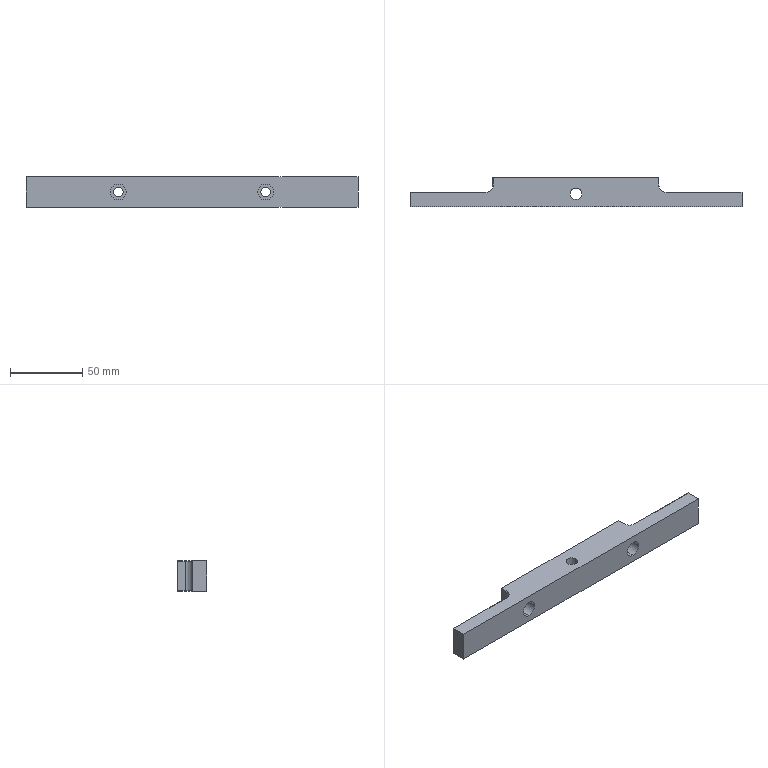Part | STEP file | 调平杆^刮墨刀-350 | 1 solid | 40 faces | box 230 x 20.5 x 21 mm | volume 70380 mm3 | plane 22 | cylinder 14 | cone 4 | commonest cylinder face diameters 6.6 x4 11 x4 3.3 x2 8 x2 10 x2
STEP:
#1=CARTESIAN_POINT('',(-51.,72.5,5.5));
#2=VERTEX_POINT('',#1);
#3=CARTESIAN_POINT('',(-51.,72.5,-5.5));
#4=VERTEX_POINT('',#3);
#5=CARTESIAN_POINT('',(-51.,72.5,0.));
#6=DIRECTION('',(0.,-1.,0.));
#7=DIRECTION('',(0.,0.,-1.));
#8=AXIS2_PLACEMENT_3D('',#5,#6,#7);
#9=CIRCLE('',#8,5.5);
#10=EDGE_CURVE('',#2,#4,#9,.T.);
#11=ORIENTED_EDGE('',*,*,#10,.F.);
#12=CARTESIAN_POINT('',(-51.,64.5,5.5));
#13=VERTEX_POINT('',#12);
#14=CARTESIAN_POINT('',(-51.,64.5,5.5));
#15=DIRECTION('',(0.,-1.,0.));
#16=VECTOR('',#15,1000.);
#17=LINE('',#14,#16);
#18=EDGE_CURVE('',#2,#13,#17,.T.);
#19=ORIENTED_EDGE('',*,*,#18,.T.);
#20=CARTESIAN_POINT('',(-51.,64.5,-5.5));
#21=VERTEX_POINT('',#20);
#22=CARTESIAN_POINT('',(-51.,64.5,0.));
#23=DIRECTION('',(0.,-1.,0.));
#24=DIRECTION('',(0.,0.,-1.));
#25=AXIS2_PLACEMENT_3D('',#22,#23,#24);
#26=CIRCLE('',#25,5.5);
#27=EDGE_CURVE('',#13,#21,#26,.T.);
#28=ORIENTED_EDGE('',*,*,#27,.T.);
#29=CARTESIAN_POINT('',(-51.,64.5,-5.5));
#30=DIRECTION('',(0.,-1.,0.));
#31=VECTOR('',#30,1000.);
#32=LINE('',#29,#31);
#33=EDGE_CURVE('',#4,#21,#32,.T.);
#34=ORIENTED_EDGE('',*,*,#33,.F.);
#35=EDGE_LOOP('',(#11,#19,#28,#34));
#36=FACE_OUTER_BOUND('',#35,.T.);
#37=CARTESIAN_POINT('',(-51.,64.5,0.));
#38=DIRECTION('',(0.,-1.,0.));
#39=DIRECTION('',(0.,0.,-1.));
#40=AXIS2_PLACEMENT_3D('',#37,#38,#39);
#41=CYLINDRICAL_SURFACE('',#40,5.5);
#42=ADVANCED_FACE('',(#36),#41,.F.);
#43=CARTESIAN_POINT('',(-51.,85.,3.3));
#44=VERTEX_POINT('',#43);
#45=CARTESIAN_POINT('',(-51.,85.,-3.3));
#46=VERTEX_POINT('',#45);
#47=CARTESIAN_POINT('',(-51.,85.,0.));
#48=DIRECTION('',(0.,-1.,0.));
#49=DIRECTION('',(0.,0.,-1.));
#50=AXIS2_PLACEMENT_3D('',#47,#48,#49);
#51=CIRCLE('',#50,3.3);
#52=EDGE_CURVE('',#44,#46,#51,.T.);
#53=ORIENTED_EDGE('',*,*,#52,.F.);
#54=CARTESIAN_POINT('',(-51.,72.5,3.3));
#55=VERTEX_POINT('',#54);
#56=CARTESIAN_POINT('',(-51.,64.5,3.3));
#57=DIRECTION('',(0.,-1.,0.));
#58=VECTOR('',#57,1000.);
#59=LINE('',#56,#58);
#60=EDGE_CURVE('',#44,#55,#59,.T.);
#61=ORIENTED_EDGE('',*,*,#60,.T.);
#62=CARTESIAN_POINT('',(-51.,72.5,-3.3));
#63=VERTEX_POINT('',#62);
#64=CARTESIAN_POINT('',(-51.,72.5,0.));
#65=DIRECTION('',(0.,-1.,0.));
#66=DIRECTION('',(0.,0.,-1.));
#67=AXIS2_PLACEMENT_3D('',#64,#65,#66);
#68=CIRCLE('',#67,3.3);
#69=EDGE_CURVE('',#55,#63,#68,.T.);
#70=ORIENTED_EDGE('',*,*,#69,.T.);
#71=CARTESIAN_POINT('',(-51.,64.5,-3.3));
#72=DIRECTION('',(0.,-1.,0.));
#73=VECTOR('',#72,1000.);
#74=LINE('',#71,#73);
#75=EDGE_CURVE('',#46,#63,#74,.T.);
#76=ORIENTED_EDGE('',*,*,#75,.F.);
#77=EDGE_LOOP('',(#53,#61,#70,#76));
#78=FACE_OUTER_BOUND('',#77,.T.);
#79=CARTESIAN_POINT('',(-51.,64.5,0.));
#80=DIRECTION('',(0.,-1.,0.));
#81=DIRECTION('',(0.,0.,-1.));
#82=AXIS2_PLACEMENT_3D('',#79,#80,#81);
#83=CYLINDRICAL_SURFACE('',#82,3.3);
#84=ADVANCED_FACE('',(#78),#83,.F.);
#85=CARTESIAN_POINT('',(51.,72.5,5.5));
#86=VERTEX_POINT('',#85);
#87=CARTESIAN_POINT('',(51.,72.5,-5.5));
#88=VERTEX_POINT('',#87);
#89=CARTESIAN_POINT('',(51.,72.5,0.));
#90=DIRECTION('',(0.,-1.,0.));
#91=DIRECTION('',(0.,0.,-1.));
#92=AXIS2_PLACEMENT_3D('',#89,#90,#91);
#93=CIRCLE('',#92,5.5);
#94=EDGE_CURVE('',#86,#88,#93,.T.);
#95=ORIENTED_EDGE('',*,*,#94,.F.);
#96=CARTESIAN_POINT('',(51.,64.5,5.5));
#97=VERTEX_POINT('',#96);
#98=CARTESIAN_POINT('',(51.,64.5,5.5));
#99=DIRECTION('',(0.,-1.,0.));
#100=VECTOR('',#99,1000.);
#101=LINE('',#98,#100);
#102=EDGE_CURVE('',#86,#97,#101,.T.);
#103=ORIENTED_EDGE('',*,*,#102,.T.);
#104=CARTESIAN_POINT('',(51.,64.5,-5.5));
#105=VERTEX_POINT('',#104);
#106=CARTESIAN_POINT('',(51.,64.5,0.));
#107=DIRECTION('',(0.,-1.,0.));
#108=DIRECTION('',(0.,0.,-1.));
#109=AXIS2_PLACEMENT_3D('',#106,#107,#108);
#110=CIRCLE('',#109,5.5);
#111=EDGE_CURVE('',#97,#105,#110,.T.);
#112=ORIENTED_EDGE('',*,*,#111,.T.);
#113=CARTESIAN_POINT('',(51.,64.5,-5.5));
#114=DIRECTION('',(0.,-1.,0.));
#115=VECTOR('',#114,1000.);
#116=LINE('',#113,#115);
#117=EDGE_CURVE('',#88,#105,#116,.T.);
#118=ORIENTED_EDGE('',*,*,#117,.F.);
#119=EDGE_LOOP('',(#95,#103,#112,#118));
#120=FACE_OUTER_BOUND('',#119,.T.);
#121=CARTESIAN_POINT('',(51.,64.5,0.));
#122=DIRECTION('',(0.,-1.,0.));
#123=DIRECTION('',(0.,0.,-1.));
#124=AXIS2_PLACEMENT_3D('',#121,#122,#123);
#125=CYLINDRICAL_SURFACE('',#124,5.5);
#126=ADVANCED_FACE('',(#120),#125,.F.);
#127=CARTESIAN_POINT('',(51.,85.,3.3));
#128=VERTEX_POINT('',#127);
#129=CARTESIAN_POINT('',(51.,85.,-3.3));
#130=VERTEX_POINT('',#129);
#131=CARTESIAN_POINT('',(51.,85.,0.));
#132=DIRECTION('',(0.,-1.,0.));
#133=DIRECTION('',(0.,0.,-1.));
#134=AXIS2_PLACEMENT_3D('',#131,#132,#133);
#135=CIRCLE('',#134,3.3);
#136=EDGE_CURVE('',#128,#130,#135,.T.);
#137=ORIENTED_EDGE('',*,*,#136,.F.);
#138=CARTESIAN_POINT('',(51.,72.5,3.3));
#139=VERTEX_POINT('',#138);
#140=CARTESIAN_POINT('',(51.,64.5,3.3));
#141=DIRECTION('',(0.,-1.,0.));
#142=VECTOR('',#141,1000.);
#143=LINE('',#140,#142);
#144=EDGE_CURVE('',#128,#139,#143,.T.);
#145=ORIENTED_EDGE('',*,*,#144,.T.);
#146=CARTESIAN_POINT('',(51.,72.5,-3.3));
#147=VERTEX_POINT('',#146);
#148=CARTESIAN_POINT('',(51.,72.5,0.));
#149=DIRECTION('',(0.,-1.,0.));
#150=DIRECTION('',(0.,0.,-1.));
#151=AXIS2_PLACEMENT_3D('',#148,#149,#150);
#152=CIRCLE('',#151,3.3);
#153=EDGE_CURVE('',#139,#147,#152,.T.);
#154=ORIENTED_EDGE('',*,*,#153,.T.);
#155=CARTESIAN_POINT('',(51.,64.5,-3.3));
#156=DIRECTION('',(0.,-1.,0.));
#157=VECTOR('',#156,1000.);
#158=LINE('',#155,#157);
#159=EDGE_CURVE('',#130,#147,#158,.T.);
#160=ORIENTED_EDGE('',*,*,#159,.F.);
#161=EDGE_LOOP('',(#137,#145,#154,#160));
#162=FACE_OUTER_BOUND('',#161,.T.);
#163=CARTESIAN_POINT('',(51.,64.5,0.));
#164=DIRECTION('',(0.,-1.,0.));
#165=DIRECTION('',(0.,0.,-1.));
#166=AXIS2_PLACEMENT_3D('',#163,#164,#165);
#167=CYLINDRICAL_SURFACE('',#166,3.3);
#168=ADVANCED_FACE('',(#162),#167,.F.);
#169=CARTESIAN_POINT('',(0.,77.5,-1.65));
#170=VERTEX_POINT('',#169);
#171=CARTESIAN_POINT('',(0.,77.5,1.65));
#172=VERTEX_POINT('',#171);
#173=CARTESIAN_POINT('',(0.,77.5,-1.65));
#174=CARTESIAN_POINT('',(-0.1086,77.5,-1.65));
#175=CARTESIAN_POINT('',(-0.2188,77.495,-1.639));
#176=CARTESIAN_POINT('',(-0.4326,77.478,-1.596));
#177=CARTESIAN_POINT('',(-0.5359,77.465,-1.564));
#178=CARTESIAN_POINT('',(-0.8355,77.417,-1.439));
#179=CARTESIAN_POINT('',(-1.016,77.372,-1.318));
#180=CARTESIAN_POINT('',(-1.244,77.303,-1.09));
#181=CARTESIAN_POINT('',(-1.311,77.28,-1.008));
#182=CARTESIAN_POINT('',(-1.43,77.236,-0.8304));
#183=CARTESIAN_POINT('',(-1.481,77.216,-0.7344));
#184=CARTESIAN_POINT('',(-1.564,77.182,-0.5355));
#185=CARTESIAN_POINT('',(-1.596,77.168,-0.4326));
#186=CARTESIAN_POINT('',(-1.639,77.149,-0.2198));
#187=CARTESIAN_POINT('',(-1.65,77.144,-0.1091));
#188=CARTESIAN_POINT('',(-1.65,77.144,0.2172));
#189=CARTESIAN_POINT('',(-1.606,77.165,0.4362));
#190=CARTESIAN_POINT('',(-1.482,77.216,0.7343));
#191=CARTESIAN_POINT('',(-1.43,77.236,0.8304));
#192=CARTESIAN_POINT('',(-1.311,77.28,1.008));
#193=CARTESIAN_POINT('',(-1.243,77.303,1.09));
#194=CARTESIAN_POINT('',(-1.092,77.349,1.242));
#195=CARTESIAN_POINT('',(-1.008,77.372,1.311));
#196=CARTESIAN_POINT('',(-0.8311,77.414,1.429));
#197=CARTESIAN_POINT('',(-0.7368,77.433,1.48));
#198=CARTESIAN_POINT('',(-0.4348,77.482,1.607));
#199=CARTESIAN_POINT('',(-0.2205,77.5,1.65));
#200=CARTESIAN_POINT('',(0.,77.5,1.65));
#201=B_SPLINE_CURVE_WITH_KNOTS('',3,(#173,#174,#175,#176,#177,#178,#179,#180,#181,#182,#183,#184,#185,#186,#187,#188,#189,#190,#191,#192,#193,#194,#195,#196,#197,#198,#199,#200),.UNSPECIFIED.,.F.,.F.,(4,2,2,2,2,2,2,2,2,2,2,2,2,4),(0.005218,0.005543,0.005869,0.006521,0.006847,0.007173,0.007499,0.007824,0.008476,0.008802,0.009128,0.009454,0.009779,0.01043),.UNSPECIFIED.);
#202=EDGE_CURVE('',#170,#172,#201,.T.);
#203=ORIENTED_EDGE('',*,*,#202,.F.);
#204=CARTESIAN_POINT('',(0.,85.,-1.65));
#205=VERTEX_POINT('',#204);
#206=CARTESIAN_POINT('',(0.,85.,-1.65));
#207=DIRECTION('',(0.,1.,0.));
#208=VECTOR('',#207,1000.);
#209=LINE('',#206,#208);
#210=EDGE_CURVE('',#170,#205,#209,.T.);
#211=ORIENTED_EDGE('',*,*,#210,.T.);
#212=CARTESIAN_POINT('',(0.,85.,1.65));
#213=VERTEX_POINT('',#212);
#214=CARTESIAN_POINT('',(0.,85.,0.));
#215=DIRECTION('',(0.,1.,0.));
#216=DIRECTION('',(0.,0.,1.));
#217=AXIS2_PLACEMENT_3D('',#214,#215,#216);
#218=CIRCLE('',#217,1.65);
#219=EDGE_CURVE('',#205,#213,#218,.T.);
#220=ORIENTED_EDGE('',*,*,#219,.T.);
#221=CARTESIAN_POINT('',(0.,85.,1.65));
#222=DIRECTION('',(0.,1.,0.));
#223=VECTOR('',#222,1000.);
#224=LINE('',#221,#223);
#225=EDGE_CURVE('',#172,#213,#224,.T.);
#226=ORIENTED_EDGE('',*,*,#225,.F.);
#227=EDGE_LOOP('',(#203,#211,#220,#226));
#228=FACE_OUTER_BOUND('',#227,.T.);
#229=CARTESIAN_POINT('',(0.,85.,0.));
#230=DIRECTION('',(0.,1.,0.));
#231=DIRECTION('',(0.,0.,1.));
#232=AXIS2_PLACEMENT_3D('',#229,#230,#231);
#233=CYLINDRICAL_SURFACE('',#232,1.65);
#234=ADVANCED_FACE('',(#228),#233,.F.);
#235=CARTESIAN_POINT('',(-4.,73.5,-10.5));
#236=VERTEX_POINT('',#235);
#237=CARTESIAN_POINT('',(4.,73.5,-10.5));
#238=VERTEX_POINT('',#237);
#239=CARTESIAN_POINT('',(0.,73.5,-10.5));
#240=DIRECTION('',(0.,0.,1.));
#241=DIRECTION('',(0.,-1.,0.));
#242=AXIS2_PLACEMENT_3D('',#239,#240,#241);
#243=CIRCLE('',#242,4.);
#244=EDGE_CURVE('',#236,#238,#243,.T.);
#245=ORIENTED_EDGE('',*,*,#244,.F.);
#246=CARTESIAN_POINT('',(-4.,73.5,10.5));
#247=VERTEX_POINT('',#246);
#248=CARTESIAN_POINT('',(-4.,73.5,-10.5));
#249=DIRECTION('',(0.,0.,1.));
#250=VECTOR('',#249,1000.);
#251=LINE('',#248,#250);
#252=EDGE_CURVE('',#236,#247,#251,.T.);
#253=ORIENTED_EDGE('',*,*,#252,.T.);
#254=CARTESIAN_POINT('',(4.,73.5,10.5));
#255=VERTEX_POINT('',#254);
#256=CARTESIAN_POINT('',(0.,73.5,10.5));
#257=DIRECTION('',(0.,0.,1.));
#258=DIRECTION('',(1.,0.,0.));
#259=AXIS2_PLACEMENT_3D('',#256,#257,#258);
#260=CIRCLE('',#259,4.);
#261=EDGE_CURVE('',#247,#255,#260,.T.);
#262=ORIENTED_EDGE('',*,*,#261,.T.);
#263=CARTESIAN_POINT('',(4.,73.5,-10.5));
#264=DIRECTION('',(0.,0.,1.));
#265=VECTOR('',#264,1000.);
#266=LINE('',#263,#265);
#267=EDGE_CURVE('',#238,#255,#266,.T.);
#268=ORIENTED_EDGE('',*,*,#267,.F.);
#269=EDGE_LOOP('',(#245,#253,#262,#268));
#270=FACE_OUTER_BOUND('',#269,.T.);
#271=CARTESIAN_POINT('',(0.,73.5,-10.5));
#272=DIRECTION('',(0.,0.,1.));
#273=DIRECTION('',(1.,0.,0.));
#274=AXIS2_PLACEMENT_3D('',#271,#272,#273);
#275=CYLINDRICAL_SURFACE('',#274,4.);
#276=ADVANCED_FACE('',(#270),#275,.F.);
#277=CARTESIAN_POINT('',(114.8,74.5,10.3));
#278=VERTEX_POINT('',#277);
#279=CARTESIAN_POINT('',(114.8,74.5,-10.3));
#280=VERTEX_POINT('',#279);
#281=CARTESIAN_POINT('',(114.8,74.5,10.5));
#282=DIRECTION('',(0.,0.,-1.));
#283=VECTOR('',#282,1000.);
#284=LINE('',#281,#283);
#285=EDGE_CURVE('',#278,#280,#284,.T.);
#286=ORIENTED_EDGE('',*,*,#285,.T.);
#287=CARTESIAN_POINT('',(62.5,74.5,-10.3));
#288=VERTEX_POINT('',#287);
#289=CARTESIAN_POINT('',(115.,74.5,-10.3));
#290=DIRECTION('',(-1.,0.,0.));
#291=VECTOR('',#290,1000.);
#292=LINE('',#289,#291);
#293=EDGE_CURVE('',#280,#288,#292,.T.);
#294=ORIENTED_EDGE('',*,*,#293,.T.);
#295=CARTESIAN_POINT('',(62.5,74.5,10.3));
#296=VERTEX_POINT('',#295);
#297=CARTESIAN_POINT('',(62.5,74.5,10.5));
#298=DIRECTION('',(0.,0.,1.));
#299=VECTOR('',#298,1000.);
#300=LINE('',#297,#299);
#301=EDGE_CURVE('',#288,#296,#300,.T.);
#302=ORIENTED_EDGE('',*,*,#301,.T.);
#303=CARTESIAN_POINT('',(115.,74.5,10.3));
#304=DIRECTION('',(1.,0.,0.));
#305=VECTOR('',#304,1000.);
#306=LINE('',#303,#305);
#307=EDGE_CURVE('',#296,#278,#306,.T.);
#308=ORIENTED_EDGE('',*,*,#307,.T.);
#309=EDGE_LOOP('',(#286,#294,#302,#308));
#310=FACE_OUTER_BOUND('',#309,.T.);
#311=CARTESIAN_POINT('',(115.,74.5,10.5));
#312=DIRECTION('',(0.,-1.,0.));
#313=DIRECTION('',(0.,0.,-1.));
#314=AXIS2_PLACEMENT_3D('',#311,#312,#313);
#315=PLANE('',#314);
#316=ADVANCED_FACE('',(#310),#315,.F.);
#317=CARTESIAN_POINT('',(-62.5,74.5,10.3));
#318=VERTEX_POINT('',#317);
#319=CARTESIAN_POINT('',(-62.5,74.5,-10.3));
#320=VERTEX_POINT('',#319);
#321=CARTESIAN_POINT('',(-62.5,74.5,-10.5));
#322=DIRECTION('',(0.,0.,-1.));
#323=VECTOR('',#322,1000.);
#324=LINE('',#321,#323);
#325=EDGE_CURVE('',#318,#320,#324,.T.);
#326=ORIENTED_EDGE('',*,*,#325,.T.);
#327=CARTESIAN_POINT('',(-114.8,74.5,-10.3));
#328=VERTEX_POINT('',#327);
#329=CARTESIAN_POINT('',(115.,74.5,-10.3));
#330=DIRECTION('',(-1.,0.,0.));
#331=VECTOR('',#330,1000.);
#332=LINE('',#329,#331);
#333=EDGE_CURVE('',#320,#328,#332,.T.);
#334=ORIENTED_EDGE('',*,*,#333,.T.);
#335=CARTESIAN_POINT('',(-114.8,74.5,10.3));
#336=VERTEX_POINT('',#335);
#337=CARTESIAN_POINT('',(-114.8,74.5,10.5));
#338=DIRECTION('',(0.,0.,1.));
#339=VECTOR('',#338,1000.);
#340=LINE('',#337,#339);
#341=EDGE_CURVE('',#328,#336,#340,.T.);
#342=ORIENTED_EDGE('',*,*,#341,.T.);
#343=CARTESIAN_POINT('',(115.,74.5,10.3));
#344=DIRECTION('',(1.,0.,0.));
#345=VECTOR('',#344,1000.);
#346=LINE('',#343,#345);
#347=EDGE_CURVE('',#336,#318,#346,.T.);
#348=ORIENTED_EDGE('',*,*,#347,.T.);
#349=EDGE_LOOP('',(#326,#334,#342,#348));
#350=FACE_OUTER_BOUND('',#349,.T.);
#351=CARTESIAN_POINT('',(115.,74.5,10.5));
#352=DIRECTION('',(0.,-1.,0.));
#353=DIRECTION('',(0.,0.,-1.));
#354=AXIS2_PLACEMENT_3D('',#351,#352,#353);
#355=PLANE('',#354);
#356=ADVANCED_FACE('',(#350),#355,.F.);
#357=CARTESIAN_POINT('',(0.,73.5,-10.5));
#358=DIRECTION('',(0.,0.,1.));
#359=DIRECTION('',(0.,-1.,0.));
#360=AXIS2_PLACEMENT_3D('',#357,#358,#359);
#361=CIRCLE('',#360,4.);
#362=EDGE_CURVE('',#238,#236,#361,.T.);
#363=ORIENTED_EDGE('',*,*,#362,.T.);
#364=ORIENTED_EDGE('',*,*,#244,.T.);
#365=EDGE_LOOP('',(#363,#364));
#366=FACE_BOUND('',#365,.T.);
#367=CARTESIAN_POINT('',(57.3,85.,-10.5));
#368=VERTEX_POINT('',#367);
#369=CARTESIAN_POINT('',(-57.3,85.,-10.5));
#370=VERTEX_POINT('',#369);
#371=CARTESIAN_POINT('',(-57.5,85.,-10.5));
#372=DIRECTION('',(-1.,0.,0.));
#373=VECTOR('',#372,1000.);
#374=LINE('',#371,#373);
#375=EDGE_CURVE('',#368,#370,#374,.T.);
#376=ORIENTED_EDGE('',*,*,#375,.F.);
#377=CARTESIAN_POINT('',(57.3,79.5,-10.5));
#378=VERTEX_POINT('',#377);
#379=CARTESIAN_POINT('',(57.3,64.5,-10.5));
#380=DIRECTION('',(0.,-1.,0.));
#381=VECTOR('',#380,1000.);
#382=LINE('',#379,#381);
#383=EDGE_CURVE('',#368,#378,#382,.T.);
#384=ORIENTED_EDGE('',*,*,#383,.T.);
#385=CARTESIAN_POINT('',(62.5,74.3,-10.5));
#386=VERTEX_POINT('',#385);
#387=CARTESIAN_POINT('',(62.5,79.5,-10.5));
#388=DIRECTION('',(0.,0.,1.));
#389=DIRECTION('',(0.,-1.,0.));
#390=AXIS2_PLACEMENT_3D('',#387,#388,#389);
#391=CIRCLE('',#390,5.2);
#392=EDGE_CURVE('',#378,#386,#391,.T.);
#393=ORIENTED_EDGE('',*,*,#392,.T.);
#394=CARTESIAN_POINT('',(115.,74.3,-10.5));
#395=VERTEX_POINT('',#394);
#396=CARTESIAN_POINT('',(115.,74.3,-10.5));
#397=DIRECTION('',(1.,0.,0.));
#398=VECTOR('',#397,1000.);
#399=LINE('',#396,#398);
#400=EDGE_CURVE('',#386,#395,#399,.T.);
#401=ORIENTED_EDGE('',*,*,#400,.T.);
#402=CARTESIAN_POINT('',(115.,64.5,-10.5));
#403=VERTEX_POINT('',#402);
#404=CARTESIAN_POINT('',(115.,64.5,-10.5));
#405=DIRECTION('',(0.,1.,0.));
#406=VECTOR('',#405,1000.);
#407=LINE('',#404,#406);
#408=EDGE_CURVE('',#403,#395,#407,.T.);
#409=ORIENTED_EDGE('',*,*,#408,.F.);
#410=CARTESIAN_POINT('',(-115.,64.5,-10.5));
#411=VERTEX_POINT('',#410);
#412=CARTESIAN_POINT('',(115.,64.5,-10.5));
#413=DIRECTION('',(-1.,0.,0.));
#414=VECTOR('',#413,1000.);
#415=LINE('',#412,#414);
#416=EDGE_CURVE('',#403,#411,#415,.T.);
#417=ORIENTED_EDGE('',*,*,#416,.T.);
#418=CARTESIAN_POINT('',(-115.,74.3,-10.5));
#419=VERTEX_POINT('',#418);
#420=CARTESIAN_POINT('',(-115.,64.5,-10.5));
#421=DIRECTION('',(0.,1.,0.));
#422=VECTOR('',#421,1000.);
#423=LINE('',#420,#422);
#424=EDGE_CURVE('',#411,#419,#423,.T.);
#425=ORIENTED_EDGE('',*,*,#424,.T.);
#426=CARTESIAN_POINT('',(-62.5,74.3,-10.5));
#427=VERTEX_POINT('',#426);
#428=CARTESIAN_POINT('',(115.,74.3,-10.5));
#429=DIRECTION('',(1.,0.,0.));
#430=VECTOR('',#429,1000.);
#431=LINE('',#428,#430);
#432=EDGE_CURVE('',#419,#427,#431,.T.);
#433=ORIENTED_EDGE('',*,*,#432,.T.);
#434=CARTESIAN_POINT('',(-57.3,79.5,-10.5));
#435=VERTEX_POINT('',#434);
#436=CARTESIAN_POINT('',(-62.5,79.5,-10.5));
#437=DIRECTION('',(0.,0.,1.));
#438=DIRECTION('',(0.,-1.,0.));
#439=AXIS2_PLACEMENT_3D('',#436,#437,#438);
#440=CIRCLE('',#439,5.2);
#441=EDGE_CURVE('',#427,#435,#440,.T.);
#442=ORIENTED_EDGE('',*,*,#441,.T.);
#443=CARTESIAN_POINT('',(-57.3,64.5,-10.5));
#444=DIRECTION('',(0.,1.,0.));
#445=VECTOR('',#444,1000.);
#446=LINE('',#443,#445);
#447=EDGE_CURVE('',#435,#370,#446,.T.);
#448=ORIENTED_EDGE('',*,*,#447,.T.);
#449=EDGE_LOOP('',(#376,#384,#393,#401,#409,#417,#425,#433,#442,#448));
#450=FACE_OUTER_BOUND('',#449,.T.);
#451=CARTESIAN_POINT('',(115.,64.5,-10.5));
#452=DIRECTION('',(0.,0.,1.));
#453=DIRECTION('',(0.,-1.,0.));
#454=AXIS2_PLACEMENT_3D('',#451,#452,#453);
#455=PLANE('',#454);
#456=ADVANCED_FACE('',(#366,#450),#455,.F.);
#457=CARTESIAN_POINT('',(0.,73.5,10.5));
#458=DIRECTION('',(0.,0.,1.));
#459=DIRECTION('',(1.,0.,0.));
#460=AXIS2_PLACEMENT_3D('',#457,#458,#459);
#461=CIRCLE('',#460,4.);
#462=EDGE_CURVE('',#255,#247,#461,.T.);
#463=ORIENTED_EDGE('',*,*,#462,.F.);
#464=ORIENTED_EDGE('',*,*,#261,.F.);
#465=EDGE_LOOP('',(#463,#464));
#466=FACE_BOUND('',#465,.T.);
#467=CARTESIAN_POINT('',(62.5,74.3,10.5));
#468=VERTEX_POINT('',#467);
#469=CARTESIAN_POINT('',(57.3,79.5,10.5));
#470=VERTEX_POINT('',#469);
#471=CARTESIAN_POINT('',(62.5,79.5,10.5));
#472=DIRECTION('',(0.,0.,-1.));
#473=DIRECTION('',(0.,1.,0.));
#474=AXIS2_PLACEMENT_3D('',#471,#472,#473);
#475=CIRCLE('',#474,5.2);
#476=EDGE_CURVE('',#468,#470,#475,.T.);
#477=ORIENTED_EDGE('',*,*,#476,.T.);
#478=CARTESIAN_POINT('',(57.3,85.,10.5));
#479=VERTEX_POINT('',#478);
#480=CARTESIAN_POINT('',(57.3,64.5,10.5));
#481=DIRECTION('',(0.,1.,0.));
#482=VECTOR('',#481,1000.);
#483=LINE('',#480,#482);
#484=EDGE_CURVE('',#470,#479,#483,.T.);
#485=ORIENTED_EDGE('',*,*,#484,.T.);
#486=CARTESIAN_POINT('',(-57.3,85.,10.5));
#487=VERTEX_POINT('',#486);
#488=CARTESIAN_POINT('',(-57.5,85.,10.5));
#489=DIRECTION('',(1.,0.,0.));
#490=VECTOR('',#489,1000.);
#491=LINE('',#488,#490);
#492=EDGE_CURVE('',#487,#479,#491,.T.);
#493=ORIENTED_EDGE('',*,*,#492,.F.);
#494=CARTESIAN_POINT('',(-57.3,79.5,10.5));
#495=VERTEX_POINT('',#494);
#496=CARTESIAN_POINT('',(-57.3,64.5,10.5));
#497=DIRECTION('',(0.,-1.,0.));
#498=VECTOR('',#497,1000.);
#499=LINE('',#496,#498);
#500=EDGE_CURVE('',#487,#495,#499,.T.);
#501=ORIENTED_EDGE('',*,*,#500,.T.);
#502=CARTESIAN_POINT('',(-62.5,74.3,10.5));
#503=VERTEX_POINT('',#502);
#504=CARTESIAN_POINT('',(-62.5,79.5,10.5));
#505=DIRECTION('',(0.,0.,-1.));
#506=DIRECTION('',(0.,1.,0.));
#507=AXIS2_PLACEMENT_3D('',#504,#505,#506);
#508=CIRCLE('',#507,5.2);
#509=EDGE_CURVE('',#495,#503,#508,.T.);
#510=ORIENTED_EDGE('',*,*,#509,.T.);
#511=CARTESIAN_POINT('',(-115.,74.3,10.5));
#512=VERTEX_POINT('',#511);
#513=CARTESIAN_POINT('',(115.,74.3,10.5));
#514=DIRECTION('',(-1.,0.,0.));
#515=VECTOR('',#514,1000.);
#516=LINE('',#513,#515);
#517=EDGE_CURVE('',#503,#512,#516,.T.);
#518=ORIENTED_EDGE('',*,*,#517,.T.);
#519=CARTESIAN_POINT('',(-115.,64.5,10.5));
#520=VERTEX_POINT('',#519);
#521=CARTESIAN_POINT('',(-115.,64.5,10.5));
#522=DIRECTION('',(0.,-1.,0.));
#523=VECTOR('',#522,1000.);
#524=LINE('',#521,#523);
#525=EDGE_CURVE('',#512,#520,#524,.T.);
#526=ORIENTED_EDGE('',*,*,#525,.T.);
#527=CARTESIAN_POINT('',(115.,64.5,10.5));
#528=VERTEX_POINT('',#527);
#529=CARTESIAN_POINT('',(115.,64.5,10.5));
#530=DIRECTION('',(-1.,0.,0.));
#531=VECTOR('',#530,1000.);
#532=LINE('',#529,#531);
#533=EDGE_CURVE('',#528,#520,#532,.T.);
#534=ORIENTED_EDGE('',*,*,#533,.F.);
#535=CARTESIAN_POINT('',(115.,74.3,10.5));
#536=VERTEX_POINT('',#535);
#537=CARTESIAN_POINT('',(115.,64.5,10.5));
#538=DIRECTION('',(0.,-1.,0.));
#539=VECTOR('',#538,1000.);
#540=LINE('',#537,#539);
#541=EDGE_CURVE('',#536,#528,#540,.T.);
#542=ORIENTED_EDGE('',*,*,#541,.F.);
#543=CARTESIAN_POINT('',(115.,74.3,10.5));
#544=DIRECTION('',(-1.,0.,0.));
#545=VECTOR('',#544,1000.);
#546=LINE('',#543,#545);
#547=EDGE_CURVE('',#536,#468,#546,.T.);
#548=ORIENTED_EDGE('',*,*,#547,.T.);
#549=EDGE_LOOP('',(#477,#485,#493,#501,#510,#518,#526,#534,#542,#548));
#550=FACE_OUTER_BOUND('',#549,.T.);
#551=CARTESIAN_POINT('',(115.,64.5,10.5));
#552=DIRECTION('',(0.,0.,-1.));
#553=DIRECTION('',(0.,1.,0.));
#554=AXIS2_PLACEMENT_3D('',#551,#552,#553);
#555=PLANE('',#554);
#556=ADVANCED_FACE('',(#466,#550),#555,.F.);
#557=CARTESIAN_POINT('',(-51.,64.5,0.));
#558=DIRECTION('',(0.,-1.,0.));
#559=DIRECTION('',(0.,0.,-1.));
#560=AXIS2_PLACEMENT_3D('',#557,#558,#559);
#561=CIRCLE('',#560,5.5);
#562=EDGE_CURVE('',#21,#13,#561,.T.);
#563=ORIENTED_EDGE('',*,*,#562,.F.);
#564=ORIENTED_EDGE('',*,*,#27,.F.);
#565=EDGE_LOOP('',(#563,#564));
#566=FACE_BOUND('',#565,.T.);
#567=CARTESIAN_POINT('',(51.,64.5,0.));
#568=DIRECTION('',(0.,-1.,0.));
#569=DIRECTION('',(0.,0.,-1.));
#570=AXIS2_PLACEMENT_3D('',#567,#568,#569);
#571=CIRCLE('',#570,5.5);
#572=EDGE_CURVE('',#105,#97,#571,.T.);
#573=ORIENTED_EDGE('',*,*,#572,.F.);
#574=ORIENTED_EDGE('',*,*,#111,.F.);
#575=EDGE_LOOP('',(#573,#574));
#576=FACE_BOUND('',#575,.T.);
#577=CARTESIAN_POINT('',(-115.,64.5,10.5));
#578=DIRECTION('',(0.,0.,-1.));
#579=VECTOR('',#578,1000.);
#580=LINE('',#577,#579);
#581=EDGE_CURVE('',#520,#411,#580,.T.);
#582=ORIENTED_EDGE('',*,*,#581,.T.);
#583=ORIENTED_EDGE('',*,*,#416,.F.);
#584=CARTESIAN_POINT('',(115.,64.5,10.5));
#585=DIRECTION('',(0.,0.,-1.));
#586=VECTOR('',#585,1000.);
#587=LINE('',#584,#586);
#588=EDGE_CURVE('',#528,#403,#587,.T.);
#589=ORIENTED_EDGE('',*,*,#588,.F.);
#590=ORIENTED_EDGE('',*,*,#533,.T.);
#591=EDGE_LOOP('',(#582,#583,#589,#590));
#592=FACE_OUTER_BOUND('',#591,.T.);
#593=CARTESIAN_POINT('',(115.,64.5,10.5));
#594=DIRECTION('',(0.,1.,0.));
#595=DIRECTION('',(0.,0.,1.));
#596=AXIS2_PLACEMENT_3D('',#593,#594,#595);
#597=PLANE('',#596);
#598=ADVANCED_FACE('',(#566,#576,#592),#597,.F.);
#599=ORIENTED_EDGE('',*,*,#408,.T.);
#600=CARTESIAN_POINT('',(115.,74.3,-10.5));
#601=DIRECTION('',(0.,0.,1.));
#602=VECTOR('',#601,1000.);
#603=LINE('',#600,#602);
#604=EDGE_CURVE('',#395,#536,#603,.T.);
#605=ORIENTED_EDGE('',*,*,#604,.T.);
#606=ORIENTED_EDGE('',*,*,#541,.T.);
#607=ORIENTED_EDGE('',*,*,#588,.T.);
#608=EDGE_LOOP('',(#599,#605,#606,#607));
#609=FACE_OUTER_BOUND('',#608,.T.);
#610=CARTESIAN_POINT('',(115.,74.5,-10.5));
#611=DIRECTION('',(-1.,0.,0.));
#612=DIRECTION('',(0.,0.,1.));
#613=AXIS2_PLACEMENT_3D('',#610,#611,#612);
#614=PLANE('',#613);
#615=ADVANCED_FACE('',(#609),#614,.F.);
#616=ORIENTED_EDGE('',*,*,#525,.F.);
#617=CARTESIAN_POINT('',(-115.,74.3,-10.5));
#618=DIRECTION('',(0.,0.,-1.));
#619=VECTOR('',#618,1000.);
#620=LINE('',#617,#619);
#621=EDGE_CURVE('',#512,#419,#620,.T.);
#622=ORIENTED_EDGE('',*,*,#621,.T.);
#623=ORIENTED_EDGE('',*,*,#424,.F.);
#624=ORIENTED_EDGE('',*,*,#581,.F.);
#625=EDGE_LOOP('',(#616,#622,#623,#624));
#626=FACE_OUTER_BOUND('',#625,.T.);
#627=CARTESIAN_POINT('',(-115.,74.5,-10.5));
#628=DIRECTION('',(-1.,0.,0.));
#629=DIRECTION('',(0.,0.,1.));
#630=AXIS2_PLACEMENT_3D('',#627,#628,#629);
#631=PLANE('',#630);
#632=ADVANCED_FACE('',(#626),#631,.T.);
#633=CARTESIAN_POINT('',(57.5,79.5,10.3));
#634=VERTEX_POINT('',#633);
#635=CARTESIAN_POINT('',(57.5,79.5,-10.3));
#636=VERTEX_POINT('',#635);
#637=CARTESIAN_POINT('',(57.5,79.5,-10.5));
#638=DIRECTION('',(0.,0.,-1.));
#639=VECTOR('',#638,1000.);
#640=LINE('',#637,#639);
#641=EDGE_CURVE('',#634,#636,#640,.T.);
#642=ORIENTED_EDGE('',*,*,#641,.T.);
#643=CARTESIAN_POINT('',(57.5,85.,-10.3));
#644=VERTEX_POINT('',#643);
#645=CARTESIAN_POINT('',(57.5,85.,-10.3));
#646=DIRECTION('',(0.,1.,0.));
#647=VECTOR('',#646,1000.);
#648=LINE('',#645,#647);
#649=EDGE_CURVE('',#636,#644,#648,.T.);
#650=ORIENTED_EDGE('',*,*,#649,.T.);
#651=CARTESIAN_POINT('',(57.5,85.,10.3));
#652=VERTEX_POINT('',#651);
#653=CARTESIAN_POINT('',(57.5,85.,10.5));
#654=DIRECTION('',(0.,0.,-1.));
#655=VECTOR('',#654,1000.);
#656=LINE('',#653,#655);
#657=EDGE_CURVE('',#652,#644,#656,.T.);
#658=ORIENTED_EDGE('',*,*,#657,.F.);
#659=CARTESIAN_POINT('',(57.5,85.,10.3));
#660=DIRECTION('',(0.,-1.,0.));
#661=VECTOR('',#660,1000.);
#662=LINE('',#659,#661);
#663=EDGE_CURVE('',#652,#634,#662,.T.);
#664=ORIENTED_EDGE('',*,*,#663,.T.);
#665=EDGE_LOOP('',(#642,#650,#658,#664));
#666=FACE_OUTER_BOUND('',#665,.T.);
#667=CARTESIAN_POINT('',(57.5,85.,10.5));
#668=DIRECTION('',(-1.,0.,0.));
#669=DIRECTION('',(0.,0.,1.));
#670=AXIS2_PLACEMENT_3D('',#667,#668,#669);
#671=PLANE('',#670);
#672=ADVANCED_FACE('',(#666),#671,.F.);
#673=CARTESIAN_POINT('',(-57.5,85.,-10.3));
#674=VERTEX_POINT('',#673);
#675=CARTESIAN_POINT('',(-57.5,85.,10.3));
#676=VERTEX_POINT('',#675);
#677=CARTESIAN_POINT('',(-57.5,85.,10.5));
#678=DIRECTION('',(0.,0.,1.));
#679=VECTOR('',#678,1000.);
#680=LINE('',#677,#679);
#681=EDGE_CURVE('',#674,#676,#680,.T.);
#682=ORIENTED_EDGE('',*,*,#681,.F.);
#683=CARTESIAN_POINT('',(-57.5,79.5,-10.3));
#684=VERTEX_POINT('',#683);
#685=CARTESIAN_POINT('',(-57.5,85.,-10.3));
#686=DIRECTION('',(0.,-1.,0.));
#687=VECTOR('',#686,1000.);
#688=LINE('',#685,#687);
#689=EDGE_CURVE('',#674,#684,#688,.T.);
#690=ORIENTED_EDGE('',*,*,#689,.T.);
#691=CARTESIAN_POINT('',(-57.5,79.5,10.3));
#692=VERTEX_POINT('',#691);
#693=CARTESIAN_POINT('',(-57.5,79.5,10.5));
#694=DIRECTION('',(0.,0.,1.));
#695=VECTOR('',#694,1000.);
#696=LINE('',#693,#695);
#697=EDGE_CURVE('',#684,#692,#696,.T.);
#698=ORIENTED_EDGE('',*,*,#697,.T.);
#699=CARTESIAN_POINT('',(-57.5,85.,10.3));
#700=DIRECTION('',(0.,1.,0.));
#701=VECTOR('',#700,1000.);
#702=LINE('',#699,#701);
#703=EDGE_CURVE('',#692,#676,#702,.T.);
#704=ORIENTED_EDGE('',*,*,#703,.T.);
#705=EDGE_LOOP('',(#682,#690,#698,#704));
#706=FACE_OUTER_BOUND('',#705,.T.);
#707=CARTESIAN_POINT('',(-57.5,85.,10.5));
#708=DIRECTION('',(1.,0.,0.));
#709=DIRECTION('',(0.,0.,-1.));
#710=AXIS2_PLACEMENT_3D('',#707,#708,#709);
#711=PLANE('',#710);
#712=ADVANCED_FACE('',(#706),#711,.F.);
#713=CARTESIAN_POINT('',(-51.,85.,0.));
#714=DIRECTION('',(0.,-1.,0.));
#715=DIRECTION('',(0.,0.,-1.));
#716=AXIS2_PLACEMENT_3D('',#713,#714,#715);
#717=CIRCLE('',#716,3.3);
#718=EDGE_CURVE('',#46,#44,#717,.T.);
#719=ORIENTED_EDGE('',*,*,#718,.T.);
#720=ORIENTED_EDGE('',*,*,#52,.T.);
#721=EDGE_LOOP('',(#719,#720));
#722=FACE_BOUND('',#721,.T.);
#723=CARTESIAN_POINT('',(51.,85.,0.));
#724=DIRECTION('',(0.,-1.,0.));
#725=DIRECTION('',(0.,0.,-1.));
#726=AXIS2_PLACEMENT_3D('',#723,#724,#725);
#727=CIRCLE('',#726,3.3);
#728=EDGE_CURVE('',#130,#128,#727,.T.);
#729=ORIENTED_EDGE('',*,*,#728,.T.);
#730=ORIENTED_EDGE('',*,*,#136,.T.);
#731=EDGE_LOOP('',(#729,#730));
#732=FACE_BOUND('',#731,.T.);
#733=CARTESIAN_POINT('',(0.,85.,0.));
#734=DIRECTION('',(0.,1.,0.));
#735=DIRECTION('',(0.,0.,1.));
#736=AXIS2_PLACEMENT_3D('',#733,#734,#735);
#737=CIRCLE('',#736,1.65);
#738=EDGE_CURVE('',#213,#205,#737,.T.);
#739=ORIENTED_EDGE('',*,*,#738,.F.);
#740=ORIENTED_EDGE('',*,*,#219,.F.);
#741=EDGE_LOOP('',(#739,#740));
#742=FACE_BOUND('',#741,.T.);
#743=ORIENTED_EDGE('',*,*,#657,.T.);
#744=CARTESIAN_POINT('',(57.3,85.,-10.5));
#745=DIRECTION('',(-0.7071,0.,-0.7071));
#746=VECTOR('',#745,1000.);
#747=LINE('',#744,#746);
#748=EDGE_CURVE('',#644,#368,#747,.T.);
#749=ORIENTED_EDGE('',*,*,#748,.T.);
#750=ORIENTED_EDGE('',*,*,#375,.T.);
#751=CARTESIAN_POINT('',(-57.5,85.,-10.3));
#752=DIRECTION('',(-0.7071,0.,0.7071));
#753=VECTOR('',#752,1000.);
#754=LINE('',#751,#753);
#755=EDGE_CURVE('',#370,#674,#754,.T.);
#756=ORIENTED_EDGE('',*,*,#755,.T.);
#757=ORIENTED_EDGE('',*,*,#681,.T.);
#758=CARTESIAN_POINT('',(-57.3,85.,10.5));
#759=DIRECTION('',(0.7071,0.,0.7071));
#760=VECTOR('',#759,1000.);
#761=LINE('',#758,#760);
#762=EDGE_CURVE('',#676,#487,#761,.T.);
#763=ORIENTED_EDGE('',*,*,#762,.T.);
#764=ORIENTED_EDGE('',*,*,#492,.T.);
#765=CARTESIAN_POINT('',(57.5,85.,10.3));
#766=DIRECTION('',(0.7071,0.,-0.7071));
#767=VECTOR('',#766,1000.);
#768=LINE('',#765,#767);
#769=EDGE_CURVE('',#479,#652,#768,.T.);
#770=ORIENTED_EDGE('',*,*,#769,.T.);
#771=EDGE_LOOP('',(#743,#749,#750,#756,#757,#763,#764,#770));
#772=FACE_OUTER_BOUND('',#771,.T.);
#773=CARTESIAN_POINT('',(57.5,85.,-10.5));
#774=DIRECTION('',(0.,-1.,0.));
#775=DIRECTION('',(0.,0.,-1.));
#776=AXIS2_PLACEMENT_3D('',#773,#774,#775);
#777=PLANE('',#776);
#778=ADVANCED_FACE('',(#722,#732,#742,#772),#777,.F.);
#779=ORIENTED_EDGE('',*,*,#252,.F.);
#780=ORIENTED_EDGE('',*,*,#362,.F.);
#781=ORIENTED_EDGE('',*,*,#267,.T.);
#782=ORIENTED_EDGE('',*,*,#462,.T.);
#783=EDGE_LOOP('',(#779,#780,#781,#782));
#784=FACE_OUTER_BOUND('',#783,.T.);
#785=CARTESIAN_POINT('',(0.,77.5,1.65));
#786=CARTESIAN_POINT('',(0.1103,77.5,1.65));
#787=CARTESIAN_POINT('',(0.2186,77.495,1.639));
#788=CARTESIAN_POINT('',(0.4313,77.478,1.596));
#789=CARTESIAN_POINT('',(0.5367,77.465,1.564));
#790=CARTESIAN_POINT('',(0.8358,77.417,1.439));
#791=CARTESIAN_POINT('',(1.017,77.372,1.316));
#792=CARTESIAN_POINT('',(1.318,77.28,1.015));
#793=CARTESIAN_POINT('',(1.44,77.233,0.8337));
#794=CARTESIAN_POINT('',(1.564,77.182,0.5367));
#795=CARTESIAN_POINT('',(1.596,77.168,0.4315));
#796=CARTESIAN_POINT('',(1.639,77.149,0.218));
#797=CARTESIAN_POINT('',(1.65,77.144,0.1101));
#798=CARTESIAN_POINT('',(1.65,77.144,-0.108));
#799=CARTESIAN_POINT('',(1.639,77.149,-0.2186));
#800=CARTESIAN_POINT('',(1.596,77.168,-0.4314));
#801=CARTESIAN_POINT('',(1.565,77.182,-0.5352));
#802=CARTESIAN_POINT('',(1.481,77.216,-0.736));
#803=CARTESIAN_POINT('',(1.43,77.236,-0.8304));
#804=CARTESIAN_POINT('',(1.311,77.28,-1.008));
#805=CARTESIAN_POINT('',(1.242,77.303,-1.092));
#806=CARTESIAN_POINT('',(1.091,77.349,-1.243));
#807=CARTESIAN_POINT('',(1.009,77.372,-1.31));
#808=CARTESIAN_POINT('',(0.8304,77.414,-1.43));
#809=CARTESIAN_POINT('',(0.7343,77.433,-1.481));
#810=CARTESIAN_POINT('',(0.4369,77.481,-1.606));
#811=CARTESIAN_POINT('',(0.2174,77.5,-1.65));
#812=CARTESIAN_POINT('',(0.,77.5,-1.65));
#813=B_SPLINE_CURVE_WITH_KNOTS('',3,(#785,#786,#787,#788,#789,#790,#791,#792,#793,#794,#795,#796,#797,#798,#799,#800,#801,#802,#803,#804,#805,#806,#807,#808,#809,#810,#811,#812),.UNSPECIFIED.,.F.,.F.,(4,2,2,2,2,2,2,2,2,2,2,2,2,4),(0.,0.0003261,0.0006522,0.001304,0.001957,0.002283,0.002609,0.002935,0.003261,0.003587,0.003913,0.004239,0.004565,0.005218),.UNSPECIFIED.);
#814=EDGE_CURVE('',#172,#170,#813,.T.);
#815=ORIENTED_EDGE('',*,*,#814,.T.);
#816=ORIENTED_EDGE('',*,*,#202,.T.);
#817=EDGE_LOOP('',(#815,#816));
#818=FACE_BOUND('',#817,.T.);
#819=CARTESIAN_POINT('',(0.,73.5,-10.5));
#820=DIRECTION('',(0.,0.,1.));
#821=DIRECTION('',(1.,0.,0.));
#822=AXIS2_PLACEMENT_3D('',#819,#820,#821);
#823=CYLINDRICAL_SURFACE('',#822,4.);
#824=ADVANCED_FACE('',(#784,#818),#823,.F.);
#825=ORIENTED_EDGE('',*,*,#301,.F.);
#826=CARTESIAN_POINT('',(62.5,79.5,-10.3));
#827=DIRECTION('',(0.,0.,-1.));
#828=DIRECTION('',(1.,0.,0.));
#829=AXIS2_PLACEMENT_3D('',#826,#827,#828);
#830=CIRCLE('',#829,5.);
#831=EDGE_CURVE('',#288,#636,#830,.T.);
#832=ORIENTED_EDGE('',*,*,#831,.T.);
#833=ORIENTED_EDGE('',*,*,#641,.F.);
#834=CARTESIAN_POINT('',(62.5,79.5,10.3));
#835=DIRECTION('',(0.,0.,1.));
#836=DIRECTION('',(-1.,0.,0.));
#837=AXIS2_PLACEMENT_3D('',#834,#835,#836);
#838=CIRCLE('',#837,5.);
#839=EDGE_CURVE('',#634,#296,#838,.T.);
#840=ORIENTED_EDGE('',*,*,#839,.T.);
#841=EDGE_LOOP('',(#825,#832,#833,#840));
#842=FACE_OUTER_BOUND('',#841,.T.);
#843=CARTESIAN_POINT('',(62.5,79.5,10.5));
#844=DIRECTION('',(0.,0.,1.));
#845=DIRECTION('',(1.,0.,0.));
#846=AXIS2_PLACEMENT_3D('',#843,#844,#845);
#847=CYLINDRICAL_SURFACE('',#846,5.);
#848=ADVANCED_FACE('',(#842),#847,.F.);
#849=ORIENTED_EDGE('',*,*,#697,.F.);
#850=CARTESIAN_POINT('',(-62.5,79.5,-10.3));
#851=DIRECTION('',(0.,0.,-1.));
#852=DIRECTION('',(1.,0.,0.));
#853=AXIS2_PLACEMENT_3D('',#850,#851,#852);
#854=CIRCLE('',#853,5.);
#855=EDGE_CURVE('',#684,#320,#854,.T.);
#856=ORIENTED_EDGE('',*,*,#855,.T.);
#857=ORIENTED_EDGE('',*,*,#325,.F.);
#858=CARTESIAN_POINT('',(-62.5,79.5,10.3));
#859=DIRECTION('',(0.,0.,1.));
#860=DIRECTION('',(-1.,0.,0.));
#861=AXIS2_PLACEMENT_3D('',#858,#859,#860);
#862=CIRCLE('',#861,5.);
#863=EDGE_CURVE('',#318,#692,#862,.T.);
#864=ORIENTED_EDGE('',*,*,#863,.T.);
#865=EDGE_LOOP('',(#849,#856,#857,#864));
#866=FACE_OUTER_BOUND('',#865,.T.);
#867=CARTESIAN_POINT('',(-62.5,79.5,10.5));
#868=DIRECTION('',(0.,0.,-1.));
#869=DIRECTION('',(-1.,0.,0.));
#870=AXIS2_PLACEMENT_3D('',#867,#868,#869);
#871=CYLINDRICAL_SURFACE('',#870,5.);
#872=ADVANCED_FACE('',(#866),#871,.F.);
#873=ORIENTED_EDGE('',*,*,#210,.F.);
#874=ORIENTED_EDGE('',*,*,#814,.F.);
#875=ORIENTED_EDGE('',*,*,#225,.T.);
#876=ORIENTED_EDGE('',*,*,#738,.T.);
#877=EDGE_LOOP('',(#873,#874,#875,#876));
#878=FACE_OUTER_BOUND('',#877,.T.);
#879=CARTESIAN_POINT('',(0.,85.,0.));
#880=DIRECTION('',(0.,1.,0.));
#881=DIRECTION('',(0.,0.,1.));
#882=AXIS2_PLACEMENT_3D('',#879,#880,#881);
#883=CYLINDRICAL_SURFACE('',#882,1.65);
#884=ADVANCED_FACE('',(#878),#883,.F.);
#885=ORIENTED_EDGE('',*,*,#144,.F.);
#886=ORIENTED_EDGE('',*,*,#728,.F.);
#887=ORIENTED_EDGE('',*,*,#159,.T.);
#888=CARTESIAN_POINT('',(51.,72.5,0.));
#889=DIRECTION('',(0.,-1.,0.));
#890=DIRECTION('',(0.,0.,-1.));
#891=AXIS2_PLACEMENT_3D('',#888,#889,#890);
#892=CIRCLE('',#891,3.3);
#893=EDGE_CURVE('',#147,#139,#892,.T.);
#894=ORIENTED_EDGE('',*,*,#893,.T.);
#895=EDGE_LOOP('',(#885,#886,#887,#894));
#896=FACE_OUTER_BOUND('',#895,.T.);
#897=CARTESIAN_POINT('',(51.,64.5,0.));
#898=DIRECTION('',(0.,-1.,0.));
#899=DIRECTION('',(0.,0.,-1.));
#900=AXIS2_PLACEMENT_3D('',#897,#898,#899);
#901=CYLINDRICAL_SURFACE('',#900,3.3);
#902=ADVANCED_FACE('',(#896),#901,.F.);
#903=ORIENTED_EDGE('',*,*,#893,.F.);
#904=ORIENTED_EDGE('',*,*,#153,.F.);
#905=EDGE_LOOP('',(#903,#904));
#906=FACE_BOUND('',#905,.T.);
#907=CARTESIAN_POINT('',(51.,72.5,0.));
#908=DIRECTION('',(0.,-1.,0.));
#909=DIRECTION('',(0.,0.,-1.));
#910=AXIS2_PLACEMENT_3D('',#907,#908,#909);
#911=CIRCLE('',#910,5.5);
#912=EDGE_CURVE('',#88,#86,#911,.T.);
#913=ORIENTED_EDGE('',*,*,#912,.T.);
#914=ORIENTED_EDGE('',*,*,#94,.T.);
#915=EDGE_LOOP('',(#913,#914));
#916=FACE_OUTER_BOUND('',#915,.T.);
#917=CARTESIAN_POINT('',(54.3,72.5,0.));
#918=DIRECTION('',(0.,1.,0.));
#919=DIRECTION('',(0.,0.,1.));
#920=AXIS2_PLACEMENT_3D('',#917,#918,#919);
#921=PLANE('',#920);
#922=ADVANCED_FACE('',(#906,#916),#921,.F.);
#923=ORIENTED_EDGE('',*,*,#102,.F.);
#924=ORIENTED_EDGE('',*,*,#912,.F.);
#925=ORIENTED_EDGE('',*,*,#117,.T.);
#926=ORIENTED_EDGE('',*,*,#572,.T.);
#927=EDGE_LOOP('',(#923,#924,#925,#926));
#928=FACE_OUTER_BOUND('',#927,.T.);
#929=CARTESIAN_POINT('',(51.,64.5,0.));
#930=DIRECTION('',(0.,-1.,0.));
#931=DIRECTION('',(0.,0.,-1.));
#932=AXIS2_PLACEMENT_3D('',#929,#930,#931);
#933=CYLINDRICAL_SURFACE('',#932,5.5);
#934=ADVANCED_FACE('',(#928),#933,.F.);
#935=ORIENTED_EDGE('',*,*,#60,.F.);
#936=ORIENTED_EDGE('',*,*,#718,.F.);
#937=ORIENTED_EDGE('',*,*,#75,.T.);
#938=CARTESIAN_POINT('',(-51.,72.5,0.));
#939=DIRECTION('',(0.,-1.,0.));
#940=DIRECTION('',(0.,0.,-1.));
#941=AXIS2_PLACEMENT_3D('',#938,#939,#940);
#942=CIRCLE('',#941,3.3);
#943=EDGE_CURVE('',#63,#55,#942,.T.);
#944=ORIENTED_EDGE('',*,*,#943,.T.);
#945=EDGE_LOOP('',(#935,#936,#937,#944));
#946=FACE_OUTER_BOUND('',#945,.T.);
#947=CARTESIAN_POINT('',(-51.,64.5,0.));
#948=DIRECTION('',(0.,-1.,0.));
#949=DIRECTION('',(0.,0.,-1.));
#950=AXIS2_PLACEMENT_3D('',#947,#948,#949);
#951=CYLINDRICAL_SURFACE('',#950,3.3);
#952=ADVANCED_FACE('',(#946),#951,.F.);
#953=ORIENTED_EDGE('',*,*,#943,.F.);
#954=ORIENTED_EDGE('',*,*,#69,.F.);
#955=EDGE_LOOP('',(#953,#954));
#956=FACE_BOUND('',#955,.T.);
#957=CARTESIAN_POINT('',(-51.,72.5,0.));
#958=DIRECTION('',(0.,-1.,0.));
#959=DIRECTION('',(0.,0.,-1.));
#960=AXIS2_PLACEMENT_3D('',#957,#958,#959);
#961=CIRCLE('',#960,5.5);
#962=EDGE_CURVE('',#4,#2,#961,.T.);
#963=ORIENTED_EDGE('',*,*,#962,.T.);
#964=ORIENTED_EDGE('',*,*,#10,.T.);
#965=EDGE_LOOP('',(#963,#964));
#966=FACE_OUTER_BOUND('',#965,.T.);
#967=CARTESIAN_POINT('',(-47.7,72.5,0.));
#968=DIRECTION('',(0.,1.,0.));
#969=DIRECTION('',(0.,0.,1.));
#970=AXIS2_PLACEMENT_3D('',#967,#968,#969);
#971=PLANE('',#970);
#972=ADVANCED_FACE('',(#956,#966),#971,.F.);
#973=ORIENTED_EDGE('',*,*,#18,.F.);
#974=ORIENTED_EDGE('',*,*,#962,.F.);
#975=ORIENTED_EDGE('',*,*,#33,.T.);
#976=ORIENTED_EDGE('',*,*,#562,.T.);
#977=EDGE_LOOP('',(#973,#974,#975,#976));
#978=FACE_OUTER_BOUND('',#977,.T.);
#979=CARTESIAN_POINT('',(-51.,64.5,0.));
#980=DIRECTION('',(0.,-1.,0.));
#981=DIRECTION('',(0.,0.,-1.));
#982=AXIS2_PLACEMENT_3D('',#979,#980,#981);
#983=CYLINDRICAL_SURFACE('',#982,5.5);
#984=ADVANCED_FACE('',(#978),#983,.F.);
#985=ORIENTED_EDGE('',*,*,#769,.F.);
#986=ORIENTED_EDGE('',*,*,#484,.F.);
#987=CARTESIAN_POINT('',(57.5,79.5,10.3));
#988=DIRECTION('',(-0.7071,0.,0.7071));
#989=VECTOR('',#988,1000.);
#990=LINE('',#987,#989);
#991=EDGE_CURVE('',#634,#470,#990,.T.);
#992=ORIENTED_EDGE('',*,*,#991,.F.);
#993=ORIENTED_EDGE('',*,*,#663,.F.);
#994=EDGE_LOOP('',(#985,#986,#992,#993));
#995=FACE_OUTER_BOUND('',#994,.T.);
#996=CARTESIAN_POINT('',(57.5,85.,10.3));
#997=DIRECTION('',(-0.7071,0.,-0.7071));
#998=DIRECTION('',(-0.7071,0.,0.7071));
#999=AXIS2_PLACEMENT_3D('',#996,#997,#998);
#1000=PLANE('',#999);
#1001=ADVANCED_FACE('',(#995),#1000,.F.);
#1002=ORIENTED_EDGE('',*,*,#991,.T.);
#1003=ORIENTED_EDGE('',*,*,#476,.F.);
#1004=CARTESIAN_POINT('',(62.5,74.5,10.3));
#1005=DIRECTION('',(0.,-0.7071,0.7071));
#1006=VECTOR('',#1005,1000.);
#1007=LINE('',#1004,#1006);
#1008=EDGE_CURVE('',#296,#468,#1007,.T.);
#1009=ORIENTED_EDGE('',*,*,#1008,.F.);
#1010=ORIENTED_EDGE('',*,*,#839,.F.);
#1011=EDGE_LOOP('',(#1002,#1003,#1009,#1010));
#1012=FACE_OUTER_BOUND('',#1011,.T.);
#1013=CARTESIAN_POINT('',(62.5,79.5,10.5));
#1014=DIRECTION('',(0.,0.,1.));
#1015=DIRECTION('',(1.,0.,0.));
#1016=AXIS2_PLACEMENT_3D('',#1013,#1014,#1015);
#1017=CONICAL_SURFACE('',#1016,5.2,0.7854);
#1018=ADVANCED_FACE('',(#1012),#1017,.F.);
#1019=ORIENTED_EDGE('',*,*,#1008,.T.);
#1020=ORIENTED_EDGE('',*,*,#547,.F.);
#1021=CARTESIAN_POINT('',(115.,74.3,10.5));
#1022=DIRECTION('',(0.5774,-0.5774,0.5774));
#1023=VECTOR('',#1022,1000.);
#1024=LINE('',#1021,#1023);
#1025=EDGE_CURVE('',#278,#536,#1024,.T.);
#1026=ORIENTED_EDGE('',*,*,#1025,.F.);
#1027=ORIENTED_EDGE('',*,*,#307,.F.);
#1028=EDGE_LOOP('',(#1019,#1020,#1026,#1027));
#1029=FACE_OUTER_BOUND('',#1028,.T.);
#1030=CARTESIAN_POINT('',(115.,74.3,10.5));
#1031=DIRECTION('',(0.,-0.7071,-0.7071));
#1032=DIRECTION('',(0.,0.7071,-0.7071));
#1033=AXIS2_PLACEMENT_3D('',#1030,#1031,#1032);
#1034=PLANE('',#1033);
#1035=ADVANCED_FACE('',(#1029),#1034,.F.);
#1036=ORIENTED_EDGE('',*,*,#1025,.T.);
#1037=ORIENTED_EDGE('',*,*,#604,.F.);
#1038=CARTESIAN_POINT('',(115.,74.3,-10.5));
#1039=DIRECTION('',(0.5774,-0.5774,-0.5774));
#1040=VECTOR('',#1039,1000.);
#1041=LINE('',#1038,#1040);
#1042=EDGE_CURVE('',#280,#395,#1041,.T.);
#1043=ORIENTED_EDGE('',*,*,#1042,.F.);
#1044=ORIENTED_EDGE('',*,*,#285,.F.);
#1045=EDGE_LOOP('',(#1036,#1037,#1043,#1044));
#1046=FACE_OUTER_BOUND('',#1045,.T.);
#1047=CARTESIAN_POINT('',(115.,74.3,-10.5));
#1048=DIRECTION('',(-0.7071,-0.7071,0.));
#1049=DIRECTION('',(0.7071,-0.7071,0.));
#1050=AXIS2_PLACEMENT_3D('',#1047,#1048,#1049);
#1051=PLANE('',#1050);
#1052=ADVANCED_FACE('',(#1046),#1051,.F.);
#1053=ORIENTED_EDGE('',*,*,#1042,.T.);
#1054=ORIENTED_EDGE('',*,*,#400,.F.);
#1055=CARTESIAN_POINT('',(62.5,74.5,-10.3));
#1056=DIRECTION('',(0.,-0.7071,-0.7071));
#1057=VECTOR('',#1056,1000.);
#1058=LINE('',#1055,#1057);
#1059=EDGE_CURVE('',#288,#386,#1058,.T.);
#1060=ORIENTED_EDGE('',*,*,#1059,.F.);
#1061=ORIENTED_EDGE('',*,*,#293,.F.);
#1062=EDGE_LOOP('',(#1053,#1054,#1060,#1061));
#1063=FACE_OUTER_BOUND('',#1062,.T.);
#1064=CARTESIAN_POINT('',(115.,74.5,-10.3));
#1065=DIRECTION('',(0.,-0.7071,0.7071));
#1066=DIRECTION('',(0.,-0.7071,-0.7071));
#1067=AXIS2_PLACEMENT_3D('',#1064,#1065,#1066);
#1068=PLANE('',#1067);
#1069=ADVANCED_FACE('',(#1063),#1068,.F.);
#1070=ORIENTED_EDGE('',*,*,#1059,.T.);
#1071=ORIENTED_EDGE('',*,*,#392,.F.);
#1072=CARTESIAN_POINT('',(57.5,79.5,-10.3));
#1073=DIRECTION('',(-0.7071,0.,-0.7071));
#1074=VECTOR('',#1073,1000.);
#1075=LINE('',#1072,#1074);
#1076=EDGE_CURVE('',#636,#378,#1075,.T.);
#1077=ORIENTED_EDGE('',*,*,#1076,.F.);
#1078=ORIENTED_EDGE('',*,*,#831,.F.);
#1079=EDGE_LOOP('',(#1070,#1071,#1077,#1078));
#1080=FACE_OUTER_BOUND('',#1079,.T.);
#1081=CARTESIAN_POINT('',(62.5,79.5,-10.5));
#1082=DIRECTION('',(0.,0.,-1.));
#1083=DIRECTION('',(-1.,0.,0.));
#1084=AXIS2_PLACEMENT_3D('',#1081,#1082,#1083);
#1085=CONICAL_SURFACE('',#1084,5.2,0.7854);
#1086=ADVANCED_FACE('',(#1080),#1085,.F.);
#1087=ORIENTED_EDGE('',*,*,#748,.F.);
#1088=ORIENTED_EDGE('',*,*,#649,.F.);
#1089=ORIENTED_EDGE('',*,*,#1076,.T.);
#1090=ORIENTED_EDGE('',*,*,#383,.F.);
#1091=EDGE_LOOP('',(#1087,#1088,#1089,#1090));
#1092=FACE_OUTER_BOUND('',#1091,.T.);
#1093=CARTESIAN_POINT('',(57.3,64.5,-10.5));
#1094=DIRECTION('',(-0.7071,0.,0.7071));
#1095=DIRECTION('',(0.7071,0.,0.7071));
#1096=AXIS2_PLACEMENT_3D('',#1093,#1094,#1095);
#1097=PLANE('',#1096);
#1098=ADVANCED_FACE('',(#1092),#1097,.F.);
#1099=ORIENTED_EDGE('',*,*,#762,.F.);
#1100=ORIENTED_EDGE('',*,*,#703,.F.);
#1101=CARTESIAN_POINT('',(-57.3,79.5,10.5));
#1102=DIRECTION('',(-0.7071,0.,-0.7071));
#1103=VECTOR('',#1102,1000.);
#1104=LINE('',#1101,#1103);
#1105=EDGE_CURVE('',#495,#692,#1104,.T.);
#1106=ORIENTED_EDGE('',*,*,#1105,.F.);
#1107=ORIENTED_EDGE('',*,*,#500,.F.);
#1108=EDGE_LOOP('',(#1099,#1100,#1106,#1107));
#1109=FACE_OUTER_BOUND('',#1108,.T.);
#1110=CARTESIAN_POINT('',(-57.3,64.5,10.5));
#1111=DIRECTION('',(0.7071,0.,-0.7071));
#1112=DIRECTION('',(-0.7071,0.,-0.7071));
#1113=AXIS2_PLACEMENT_3D('',#1110,#1111,#1112);
#1114=PLANE('',#1113);
#1115=ADVANCED_FACE('',(#1109),#1114,.F.);
#1116=ORIENTED_EDGE('',*,*,#1105,.T.);
#1117=ORIENTED_EDGE('',*,*,#863,.F.);
#1118=CARTESIAN_POINT('',(-62.5,74.3,10.5));
#1119=DIRECTION('',(0.,0.7071,-0.7071));
#1120=VECTOR('',#1119,1000.);
#1121=LINE('',#1118,#1120);
#1122=EDGE_CURVE('',#503,#318,#1121,.T.);
#1123=ORIENTED_EDGE('',*,*,#1122,.F.);
#1124=ORIENTED_EDGE('',*,*,#509,.F.);
#1125=EDGE_LOOP('',(#1116,#1117,#1123,#1124));
#1126=FACE_OUTER_BOUND('',#1125,.T.);
#1127=CARTESIAN_POINT('',(-62.5,79.5,10.5));
#1128=DIRECTION('',(0.,0.,1.));
#1129=DIRECTION('',(1.,0.,0.));
#1130=AXIS2_PLACEMENT_3D('',#1127,#1128,#1129);
#1131=CONICAL_SURFACE('',#1130,5.2,0.7854);
#1132=ADVANCED_FACE('',(#1126),#1131,.F.);
#1133=ORIENTED_EDGE('',*,*,#1122,.T.);
#1134=ORIENTED_EDGE('',*,*,#347,.F.);
#1135=CARTESIAN_POINT('',(-38.333,150.967,-66.167));
#1136=DIRECTION('',(0.5774,0.5774,-0.5774));
#1137=VECTOR('',#1136,1000.);
#1138=LINE('',#1135,#1137);
#1139=EDGE_CURVE('',#512,#336,#1138,.T.);
#1140=ORIENTED_EDGE('',*,*,#1139,.F.);
#1141=ORIENTED_EDGE('',*,*,#517,.F.);
#1142=EDGE_LOOP('',(#1133,#1134,#1140,#1141));
#1143=FACE_OUTER_BOUND('',#1142,.T.);
#1144=CARTESIAN_POINT('',(115.,74.3,10.5));
#1145=DIRECTION('',(0.,-0.7071,-0.7071));
#1146=DIRECTION('',(0.,0.7071,-0.7071));
#1147=AXIS2_PLACEMENT_3D('',#1144,#1145,#1146);
#1148=PLANE('',#1147);
#1149=ADVANCED_FACE('',(#1143),#1148,.F.);
#1150=ORIENTED_EDGE('',*,*,#1139,.T.);
#1151=ORIENTED_EDGE('',*,*,#341,.F.);
#1152=CARTESIAN_POINT('',(-38.2,151.1,66.3));
#1153=DIRECTION('',(0.5774,0.5774,0.5774));
#1154=VECTOR('',#1153,1000.);
#1155=LINE('',#1152,#1154);
#1156=EDGE_CURVE('',#419,#328,#1155,.T.);
#1157=ORIENTED_EDGE('',*,*,#1156,.F.);
#1158=ORIENTED_EDGE('',*,*,#621,.F.);
#1159=EDGE_LOOP('',(#1150,#1151,#1157,#1158));
#1160=FACE_OUTER_BOUND('',#1159,.T.);
#1161=CARTESIAN_POINT('',(-114.8,74.5,10.5));
#1162=DIRECTION('',(-0.7071,0.7071,0.));
#1163=DIRECTION('',(-0.7071,-0.7071,0.));
#1164=AXIS2_PLACEMENT_3D('',#1161,#1162,#1163);
#1165=PLANE('',#1164);
#1166=ADVANCED_FACE('',(#1160),#1165,.T.);
#1167=ORIENTED_EDGE('',*,*,#1156,.T.);
#1168=ORIENTED_EDGE('',*,*,#333,.F.);
#1169=CARTESIAN_POINT('',(-62.5,74.3,-10.5));
#1170=DIRECTION('',(0.,0.7071,0.7071));
#1171=VECTOR('',#1170,1000.);
#1172=LINE('',#1169,#1171);
#1173=EDGE_CURVE('',#427,#320,#1172,.T.);
#1174=ORIENTED_EDGE('',*,*,#1173,.F.);
#1175=ORIENTED_EDGE('',*,*,#432,.F.);
#1176=EDGE_LOOP('',(#1167,#1168,#1174,#1175));
#1177=FACE_OUTER_BOUND('',#1176,.T.);
#1178=CARTESIAN_POINT('',(115.,74.5,-10.3));
#1179=DIRECTION('',(0.,-0.7071,0.7071));
#1180=DIRECTION('',(0.,-0.7071,-0.7071));
#1181=AXIS2_PLACEMENT_3D('',#1178,#1179,#1180);
#1182=PLANE('',#1181);
#1183=ADVANCED_FACE('',(#1177),#1182,.F.);
#1184=ORIENTED_EDGE('',*,*,#1173,.T.);
#1185=ORIENTED_EDGE('',*,*,#855,.F.);
#1186=CARTESIAN_POINT('',(-57.3,79.5,-10.5));
#1187=DIRECTION('',(-0.7071,0.,0.7071));
#1188=VECTOR('',#1187,1000.);
#1189=LINE('',#1186,#1188);
#1190=EDGE_CURVE('',#435,#684,#1189,.T.);
#1191=ORIENTED_EDGE('',*,*,#1190,.F.);
#1192=ORIENTED_EDGE('',*,*,#441,.F.);
#1193=EDGE_LOOP('',(#1184,#1185,#1191,#1192));
#1194=FACE_OUTER_BOUND('',#1193,.T.);
#1195=CARTESIAN_POINT('',(-62.5,79.5,-10.5));
#1196=DIRECTION('',(0.,0.,-1.));
#1197=DIRECTION('',(-1.,0.,0.));
#1198=AXIS2_PLACEMENT_3D('',#1195,#1196,#1197);
#1199=CONICAL_SURFACE('',#1198,5.2,0.7854);
#1200=ADVANCED_FACE('',(#1194),#1199,.F.);
#1201=ORIENTED_EDGE('',*,*,#755,.F.);
#1202=ORIENTED_EDGE('',*,*,#447,.F.);
#1203=ORIENTED_EDGE('',*,*,#1190,.T.);
#1204=ORIENTED_EDGE('',*,*,#689,.F.);
#1205=EDGE_LOOP('',(#1201,#1202,#1203,#1204));
#1206=FACE_OUTER_BOUND('',#1205,.T.);
#1207=CARTESIAN_POINT('',(-57.5,85.,-10.3));
#1208=DIRECTION('',(0.7071,0.,0.7071));
#1209=DIRECTION('',(0.7071,0.,-0.7071));
#1210=AXIS2_PLACEMENT_3D('',#1207,#1208,#1209);
#1211=PLANE('',#1210);
#1212=ADVANCED_FACE('',(#1206),#1211,.F.);
#1213=CLOSED_SHELL('',(#42,#84,#126,#168,#234,#276,#316,#356,#456,#556,#598,#615,#632,#672,#712,#778,#824,#848,#872,#884,#902,#922,#934,#952,#972,#984,#1001,#1018,#1035,#1052,#1069,#1086,#1098,#1115,#1132,#1149,#1166,#1183,#1200,#1212));
#1214=MANIFOLD_SOLID_BREP('',#1213);
#1215=CARTESIAN_POINT('',(0.,0.,0.));
#1216=DIRECTION('',(0.,0.,1.));
#1217=DIRECTION('',(1.,0.,0.));
#1218=AXIS2_PLACEMENT_3D('',#1215,#1216,#1217);
#1219=(LENGTH_UNIT()NAMED_UNIT(*)SI_UNIT(.MILLI.,.METRE.));
#1220=UNCERTAINTY_MEASURE_WITH_UNIT(LENGTH_MEASURE(0.00001),#1219,'','');
#1221=(NAMED_UNIT(*)PLANE_ANGLE_UNIT()SI_UNIT($,.RADIAN.));
#1222=(NAMED_UNIT(*)SI_UNIT($,.STERADIAN.)SOLID_ANGLE_UNIT());
#1223=(GEOMETRIC_REPRESENTATION_CONTEXT(3)GLOBAL_UNCERTAINTY_ASSIGNED_CONTEXT((#1220))GLOBAL_UNIT_ASSIGNED_CONTEXT((#1219,#1221,#1222))REPRESENTATION_CONTEXT('',''));
#1224=ADVANCED_BREP_SHAPE_REPRESENTATION('',(#1214,#1218),#1223);